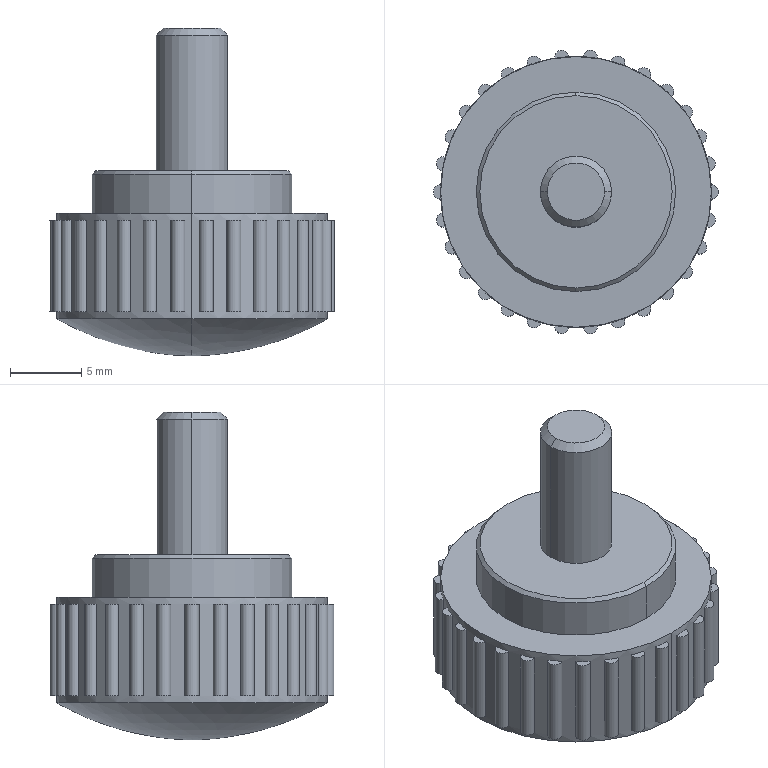Part | STEP file | HAU61-M5-L15^power cover plate | 1 solid | 120 faces | box 20 x 19.896 x 23 mm | volume 3201 mm3 | plane 63 | cylinder 51 | cone 4 | spline 2 | commonest cylinder face diameters 1 x45 5 x2 14 x2 19 x2